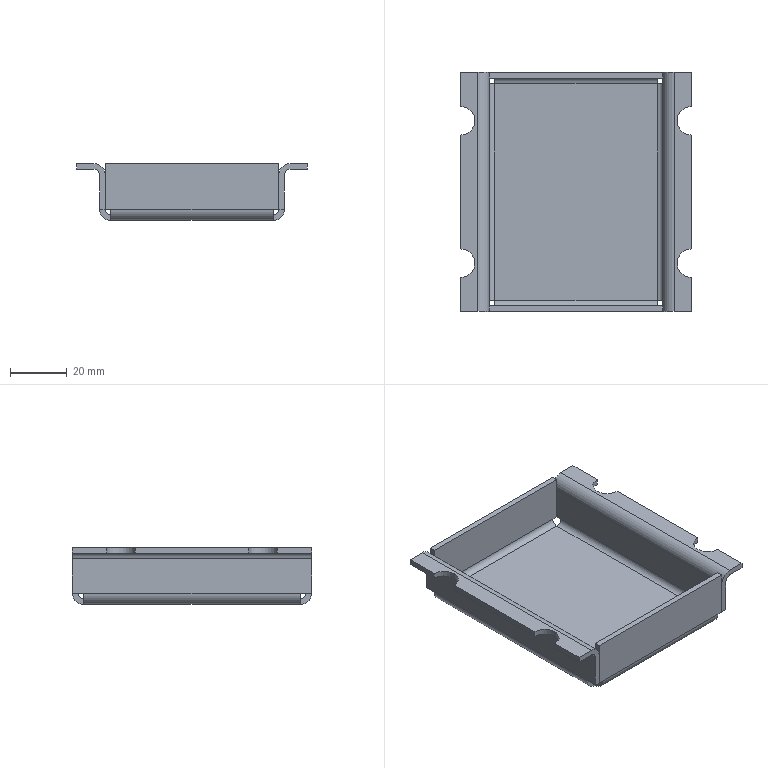Part | NX | features solid 2 | 1 solid | 62 faces | box 81 x 84 x 20 mm | volume 22379 mm3 | plane 46 | cylinder 16 | commonest cylinder face diameters 4 x6 8 x6 10 x4